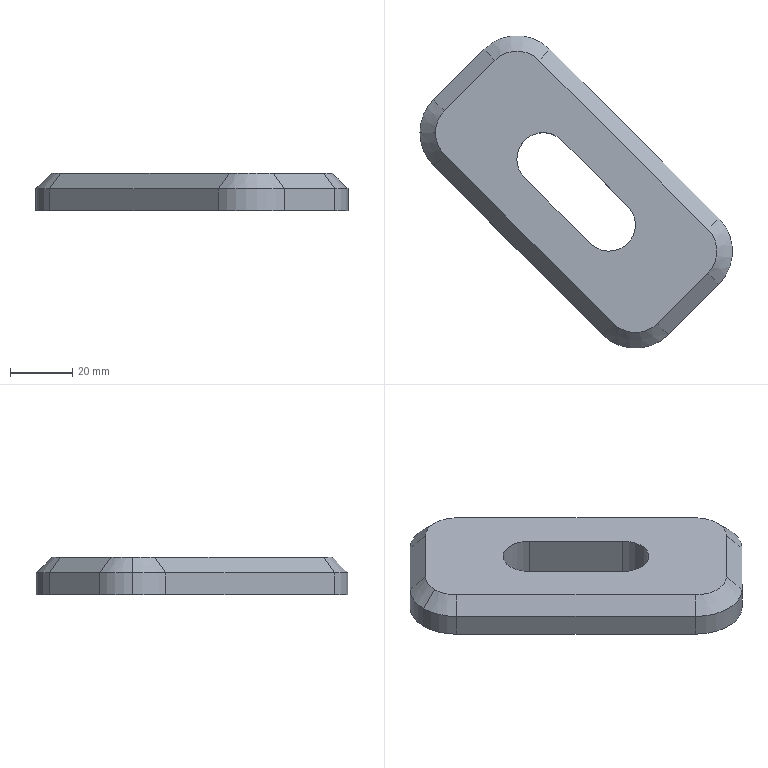Part | SolidWorks | features Chamfer 1, FlatPattern 1, SMBaseFlange 1, SheetMetal 1 | 1 solid | 25 faces | box 100.711 x 100.711 x 12 mm | volume 53343 mm3 | plane 12 | cylinder 8 | cone 5 | commonest cylinder face diameters 30 x5 17 x3
STEP:
#1=CARTESIAN_POINT('',(-96.355,309.376,12.));
#2=VERTEX_POINT('',#1);
#3=CARTESIAN_POINT('',(-93.426,302.305,12.));
#4=VERTEX_POINT('',#3);
#5=CARTESIAN_POINT('',(-86.355,309.376,12.));
#6=DIRECTION('',(0.,0.,1.));
#7=DIRECTION('',(-1.,0.,0.));
#8=AXIS2_PLACEMENT_3D('',#5,#6,#7);
#9=CIRCLE('',#8,10.);
#10=EDGE_CURVE('',#2,#4,#9,.T.);
#11=ORIENTED_EDGE('',*,*,#10,.F.);
#12=CARTESIAN_POINT('',(-101.355,309.376,7.));
#13=VERTEX_POINT('',#12);
#14=CARTESIAN_POINT('',(-96.355,309.376,12.));
#15=DIRECTION('',(-0.7071,0.,-0.7071));
#16=VECTOR('',#15,1000.);
#17=LINE('',#14,#16);
#18=EDGE_CURVE('',#2,#13,#17,.T.);
#19=ORIENTED_EDGE('',*,*,#18,.T.);
#20=CARTESIAN_POINT('',(-96.962,298.77,7.));
#21=VERTEX_POINT('',#20);
#22=CARTESIAN_POINT('',(-86.355,309.376,7.));
#23=DIRECTION('',(0.,0.,-1.));
#24=DIRECTION('',(-1.,0.,0.));
#25=AXIS2_PLACEMENT_3D('',#22,#23,#24);
#26=CIRCLE('',#25,15.);
#27=EDGE_CURVE('',#21,#13,#26,.T.);
#28=ORIENTED_EDGE('',*,*,#27,.F.);
#29=CARTESIAN_POINT('',(-96.962,298.77,7.));
#30=DIRECTION('',(0.5,0.5,0.7071));
#31=VECTOR('',#30,1000.);
#32=LINE('',#29,#31);
#33=EDGE_CURVE('',#21,#4,#32,.T.);
#34=ORIENTED_EDGE('',*,*,#33,.T.);
#35=EDGE_LOOP('',(#11,#19,#28,#34));
#36=FACE_OUTER_BOUND('',#35,.T.);
#37=CARTESIAN_POINT('',(-86.355,309.376,12.));
#38=DIRECTION('',(0.,0.,-1.));
#39=DIRECTION('',(-1.,0.,0.));
#40=AXIS2_PLACEMENT_3D('',#37,#38,#39);
#41=CONICAL_SURFACE('',#40,10.,0.7854);
#42=ADVANCED_FACE('',(#36),#41,.T.);
#43=CARTESIAN_POINT('',(-55.596,306.901,12.));
#44=VERTEX_POINT('',#43);
#45=CARTESIAN_POINT('',(-70.107,300.891,12.));
#46=VERTEX_POINT('',#45);
#47=CARTESIAN_POINT('',(-61.607,300.891,12.));
#48=DIRECTION('',(0.,0.,1.));
#49=DIRECTION('',(1.,0.,0.));
#50=AXIS2_PLACEMENT_3D('',#47,#48,#49);
#51=CIRCLE('',#50,8.5);
#52=EDGE_CURVE('',#44,#46,#51,.T.);
#53=ORIENTED_EDGE('',*,*,#52,.T.);
#54=CARTESIAN_POINT('',(-70.107,300.891,0.));
#55=VERTEX_POINT('',#54);
#56=CARTESIAN_POINT('',(-70.107,300.891,12.));
#57=DIRECTION('',(0.,0.,-1.));
#58=VECTOR('',#57,1000.);
#59=LINE('',#56,#58);
#60=EDGE_CURVE('',#46,#55,#59,.T.);
#61=ORIENTED_EDGE('',*,*,#60,.T.);
#62=CARTESIAN_POINT('',(-55.596,306.901,0.));
#63=VERTEX_POINT('',#62);
#64=CARTESIAN_POINT('',(-61.607,300.891,0.));
#65=DIRECTION('',(0.,0.,1.));
#66=DIRECTION('',(1.,0.,0.));
#67=AXIS2_PLACEMENT_3D('',#64,#65,#66);
#68=CIRCLE('',#67,8.5);
#69=EDGE_CURVE('',#63,#55,#68,.T.);
#70=ORIENTED_EDGE('',*,*,#69,.F.);
#71=CARTESIAN_POINT('',(-55.596,306.901,12.));
#72=DIRECTION('',(0.,0.,-1.));
#73=VECTOR('',#72,1000.);
#74=LINE('',#71,#73);
#75=EDGE_CURVE('',#44,#63,#74,.T.);
#76=ORIENTED_EDGE('',*,*,#75,.F.);
#77=EDGE_LOOP('',(#53,#61,#70,#76));
#78=FACE_OUTER_BOUND('',#77,.T.);
#79=CARTESIAN_POINT('',(-61.607,300.891,12.));
#80=DIRECTION('',(0.,0.,-1.));
#81=DIRECTION('',(-1.,0.,0.));
#82=AXIS2_PLACEMENT_3D('',#79,#80,#81);
#83=CYLINDRICAL_SURFACE('',#82,8.5);
#84=ADVANCED_FACE('',(#78),#83,.F.);
#85=ORIENTED_EDGE('',*,*,#27,.T.);
#86=CARTESIAN_POINT('',(-101.355,309.376,0.));
#87=VERTEX_POINT('',#86);
#88=CARTESIAN_POINT('',(-101.355,309.376,12.));
#89=DIRECTION('',(0.,0.,-1.));
#90=VECTOR('',#89,1000.);
#91=LINE('',#88,#90);
#92=EDGE_CURVE('',#13,#87,#91,.T.);
#93=ORIENTED_EDGE('',*,*,#92,.T.);
#94=CARTESIAN_POINT('',(-96.962,298.77,0.));
#95=VERTEX_POINT('',#94);
#96=CARTESIAN_POINT('',(-86.355,309.376,0.));
#97=DIRECTION('',(0.,0.,1.));
#98=DIRECTION('',(-1.,0.,0.));
#99=AXIS2_PLACEMENT_3D('',#96,#97,#98);
#100=CIRCLE('',#99,15.);
#101=EDGE_CURVE('',#87,#95,#100,.T.);
#102=ORIENTED_EDGE('',*,*,#101,.T.);
#103=CARTESIAN_POINT('',(-96.962,298.77,12.));
#104=DIRECTION('',(0.,0.,-1.));
#105=VECTOR('',#104,1000.);
#106=LINE('',#103,#105);
#107=EDGE_CURVE('',#21,#95,#106,.T.);
#108=ORIENTED_EDGE('',*,*,#107,.F.);
#109=EDGE_LOOP('',(#85,#93,#102,#108));
#110=FACE_OUTER_BOUND('',#109,.T.);
#111=CARTESIAN_POINT('',(-86.355,309.376,12.));
#112=DIRECTION('',(0.,0.,-1.));
#113=DIRECTION('',(-1.,0.,0.));
#114=AXIS2_PLACEMENT_3D('',#111,#112,#113);
#115=CYLINDRICAL_SURFACE('',#114,15.);
#116=ADVANCED_FACE('',(#110),#115,.T.);
#117=CARTESIAN_POINT('',(-8.574,264.121,12.));
#118=VERTEX_POINT('',#117);
#119=CARTESIAN_POINT('',(-8.574,278.263,12.));
#120=VERTEX_POINT('',#119);
#121=CARTESIAN_POINT('',(-15.645,271.192,12.));
#122=DIRECTION('',(0.,0.,1.));
#123=DIRECTION('',(-1.,0.,0.));
#124=AXIS2_PLACEMENT_3D('',#121,#122,#123);
#125=CIRCLE('',#124,10.);
#126=EDGE_CURVE('',#118,#120,#125,.T.);
#127=ORIENTED_EDGE('',*,*,#126,.T.);
#128=CARTESIAN_POINT('',(-63.021,332.711,12.));
#129=VERTEX_POINT('',#128);
#130=CARTESIAN_POINT('',(-8.574,278.263,12.));
#131=DIRECTION('',(-0.7071,0.7071,0.));
#132=VECTOR('',#131,1000.);
#133=LINE('',#130,#132);
#134=EDGE_CURVE('',#120,#129,#133,.T.);
#135=ORIENTED_EDGE('',*,*,#134,.T.);
#136=CARTESIAN_POINT('',(-77.163,332.711,12.));
#137=VERTEX_POINT('',#136);
#138=CARTESIAN_POINT('',(-70.092,325.64,12.));
#139=DIRECTION('',(0.,0.,1.));
#140=DIRECTION('',(-1.,0.,0.));
#141=AXIS2_PLACEMENT_3D('',#138,#139,#140);
#142=CIRCLE('',#141,10.);
#143=EDGE_CURVE('',#129,#137,#142,.T.);
#144=ORIENTED_EDGE('',*,*,#143,.T.);
#145=CARTESIAN_POINT('',(-93.426,316.447,12.));
#146=VERTEX_POINT('',#145);
#147=CARTESIAN_POINT('',(-77.163,332.711,12.));
#148=DIRECTION('',(-0.7071,-0.7071,0.));
#149=VECTOR('',#148,1000.);
#150=LINE('',#147,#149);
#151=EDGE_CURVE('',#137,#146,#150,.T.);
#152=ORIENTED_EDGE('',*,*,#151,.T.);
#153=CARTESIAN_POINT('',(-86.355,309.376,12.));
#154=DIRECTION('',(0.,0.,1.));
#155=DIRECTION('',(-1.,0.,0.));
#156=AXIS2_PLACEMENT_3D('',#153,#154,#155);
#157=CIRCLE('',#156,10.);
#158=EDGE_CURVE('',#146,#2,#157,.T.);
#159=ORIENTED_EDGE('',*,*,#158,.T.);
#160=ORIENTED_EDGE('',*,*,#10,.T.);
#161=CARTESIAN_POINT('',(-38.979,247.858,12.));
#162=VERTEX_POINT('',#161);
#163=CARTESIAN_POINT('',(-38.979,247.858,12.));
#164=DIRECTION('',(0.7071,-0.7071,0.));
#165=VECTOR('',#164,1000.);
#166=LINE('',#163,#165);
#167=EDGE_CURVE('',#4,#162,#166,.T.);
#168=ORIENTED_EDGE('',*,*,#167,.T.);
#169=CARTESIAN_POINT('',(-24.837,247.858,12.));
#170=VERTEX_POINT('',#169);
#171=CARTESIAN_POINT('',(-31.908,254.929,12.));
#172=DIRECTION('',(0.,0.,1.));
#173=DIRECTION('',(-1.,0.,0.));
#174=AXIS2_PLACEMENT_3D('',#171,#172,#173);
#175=CIRCLE('',#174,10.);
#176=EDGE_CURVE('',#162,#170,#175,.T.);
#177=ORIENTED_EDGE('',*,*,#176,.T.);
#178=CARTESIAN_POINT('',(-8.574,264.121,12.));
#179=DIRECTION('',(0.7071,0.7071,0.));
#180=VECTOR('',#179,1000.);
#181=LINE('',#178,#180);
#182=EDGE_CURVE('',#170,#118,#181,.T.);
#183=ORIENTED_EDGE('',*,*,#182,.T.);
#184=EDGE_LOOP('',(#127,#135,#144,#152,#159,#160,#168,#177,#183));
#185=FACE_OUTER_BOUND('',#184,.T.);
#186=CARTESIAN_POINT('',(-46.404,273.667,12.));
#187=VERTEX_POINT('',#186);
#188=CARTESIAN_POINT('',(-34.383,285.688,12.));
#189=VERTEX_POINT('',#188);
#190=CARTESIAN_POINT('',(-40.393,279.678,12.));
#191=DIRECTION('',(0.,0.,1.));
#192=DIRECTION('',(1.,0.,0.));
#193=AXIS2_PLACEMENT_3D('',#190,#191,#192);
#194=CIRCLE('',#193,8.5);
#195=EDGE_CURVE('',#187,#189,#194,.T.);
#196=ORIENTED_EDGE('',*,*,#195,.F.);
#197=CARTESIAN_POINT('',(-67.617,294.88,12.));
#198=VERTEX_POINT('',#197);
#199=CARTESIAN_POINT('',(-46.404,273.667,12.));
#200=DIRECTION('',(0.7071,-0.7071,0.));
#201=VECTOR('',#200,1000.);
#202=LINE('',#199,#201);
#203=EDGE_CURVE('',#198,#187,#202,.T.);
#204=ORIENTED_EDGE('',*,*,#203,.F.);
#205=CARTESIAN_POINT('',(-61.607,300.891,12.));
#206=DIRECTION('',(0.,0.,1.));
#207=DIRECTION('',(1.,0.,0.));
#208=AXIS2_PLACEMENT_3D('',#205,#206,#207);
#209=CIRCLE('',#208,8.5);
#210=EDGE_CURVE('',#46,#198,#209,.T.);
#211=ORIENTED_EDGE('',*,*,#210,.F.);
#212=ORIENTED_EDGE('',*,*,#52,.F.);
#213=CARTESIAN_POINT('',(-34.383,285.688,12.));
#214=DIRECTION('',(-0.7071,0.7071,0.));
#215=VECTOR('',#214,1000.);
#216=LINE('',#213,#215);
#217=EDGE_CURVE('',#189,#44,#216,.T.);
#218=ORIENTED_EDGE('',*,*,#217,.F.);
#219=EDGE_LOOP('',(#196,#204,#211,#212,#218));
#220=FACE_BOUND('',#219,.T.);
#221=CARTESIAN_POINT('',(-15.645,271.192,12.));
#222=DIRECTION('',(0.,0.,-1.));
#223=DIRECTION('',(-1.,0.,0.));
#224=AXIS2_PLACEMENT_3D('',#221,#222,#223);
#225=PLANE('',#224);
#226=ADVANCED_FACE('',(#185,#220),#225,.F.);
#227=CARTESIAN_POINT('',(-5.038,260.586,0.));
#228=VERTEX_POINT('',#227);
#229=CARTESIAN_POINT('',(-5.038,281.799,0.));
#230=VERTEX_POINT('',#229);
#231=CARTESIAN_POINT('',(-15.645,271.192,0.));
#232=DIRECTION('',(0.,0.,1.));
#233=DIRECTION('',(-1.,0.,0.));
#234=AXIS2_PLACEMENT_3D('',#231,#232,#233);
#235=CIRCLE('',#234,15.);
#236=EDGE_CURVE('',#228,#230,#235,.T.);
#237=ORIENTED_EDGE('',*,*,#236,.F.);
#238=CARTESIAN_POINT('',(-21.302,244.322,0.));
#239=VERTEX_POINT('',#238);
#240=CARTESIAN_POINT('',(-5.038,260.586,0.));
#241=DIRECTION('',(0.7071,0.7071,0.));
#242=VECTOR('',#241,1000.);
#243=LINE('',#240,#242);
#244=EDGE_CURVE('',#239,#228,#243,.T.);
#245=ORIENTED_EDGE('',*,*,#244,.F.);
#246=CARTESIAN_POINT('',(-42.515,244.322,0.));
#247=VERTEX_POINT('',#246);
#248=CARTESIAN_POINT('',(-31.908,254.929,0.));
#249=DIRECTION('',(0.,0.,1.));
#250=DIRECTION('',(-1.,0.,0.));
#251=AXIS2_PLACEMENT_3D('',#248,#249,#250);
#252=CIRCLE('',#251,15.);
#253=EDGE_CURVE('',#247,#239,#252,.T.);
#254=ORIENTED_EDGE('',*,*,#253,.F.);
#255=CARTESIAN_POINT('',(-42.515,244.322,0.));
#256=DIRECTION('',(0.7071,-0.7071,0.));
#257=VECTOR('',#256,1000.);
#258=LINE('',#255,#257);
#259=EDGE_CURVE('',#95,#247,#258,.T.);
#260=ORIENTED_EDGE('',*,*,#259,.F.);
#261=ORIENTED_EDGE('',*,*,#101,.F.);
#262=CARTESIAN_POINT('',(-96.962,319.983,0.));
#263=VERTEX_POINT('',#262);
#264=CARTESIAN_POINT('',(-86.355,309.376,0.));
#265=DIRECTION('',(0.,0.,1.));
#266=DIRECTION('',(-1.,0.,0.));
#267=AXIS2_PLACEMENT_3D('',#264,#265,#266);
#268=CIRCLE('',#267,15.);
#269=EDGE_CURVE('',#263,#87,#268,.T.);
#270=ORIENTED_EDGE('',*,*,#269,.F.);
#271=CARTESIAN_POINT('',(-80.698,336.246,0.));
#272=VERTEX_POINT('',#271);
#273=CARTESIAN_POINT('',(-96.962,319.983,0.));
#274=DIRECTION('',(-0.7071,-0.7071,0.));
#275=VECTOR('',#274,1000.);
#276=LINE('',#273,#275);
#277=EDGE_CURVE('',#272,#263,#276,.T.);
#278=ORIENTED_EDGE('',*,*,#277,.F.);
#279=CARTESIAN_POINT('',(-59.485,336.246,0.));
#280=VERTEX_POINT('',#279);
#281=CARTESIAN_POINT('',(-70.092,325.64,0.));
#282=DIRECTION('',(0.,0.,1.));
#283=DIRECTION('',(1.,0.,0.));
#284=AXIS2_PLACEMENT_3D('',#281,#282,#283);
#285=CIRCLE('',#284,15.);
#286=EDGE_CURVE('',#280,#272,#285,.T.);
#287=ORIENTED_EDGE('',*,*,#286,.F.);
#288=CARTESIAN_POINT('',(-59.485,336.246,0.));
#289=DIRECTION('',(-0.7071,0.7071,0.));
#290=VECTOR('',#289,1000.);
#291=LINE('',#288,#290);
#292=EDGE_CURVE('',#230,#280,#291,.T.);
#293=ORIENTED_EDGE('',*,*,#292,.F.);
#294=EDGE_LOOP('',(#237,#245,#254,#260,#261,#270,#278,#287,#293));
#295=FACE_OUTER_BOUND('',#294,.T.);
#296=CARTESIAN_POINT('',(-67.617,294.88,0.));
#297=VERTEX_POINT('',#296);
#298=CARTESIAN_POINT('',(-46.404,273.667,0.));
#299=VERTEX_POINT('',#298);
#300=CARTESIAN_POINT('',(-46.404,273.667,0.));
#301=DIRECTION('',(0.7071,-0.7071,0.));
#302=VECTOR('',#301,1000.);
#303=LINE('',#300,#302);
#304=EDGE_CURVE('',#297,#299,#303,.T.);
#305=ORIENTED_EDGE('',*,*,#304,.T.);
#306=CARTESIAN_POINT('',(-34.383,285.688,0.));
#307=VERTEX_POINT('',#306);
#308=CARTESIAN_POINT('',(-40.393,279.678,0.));
#309=DIRECTION('',(0.,0.,1.));
#310=DIRECTION('',(1.,0.,0.));
#311=AXIS2_PLACEMENT_3D('',#308,#309,#310);
#312=CIRCLE('',#311,8.5);
#313=EDGE_CURVE('',#299,#307,#312,.T.);
#314=ORIENTED_EDGE('',*,*,#313,.T.);
#315=CARTESIAN_POINT('',(-34.383,285.688,0.));
#316=DIRECTION('',(-0.7071,0.7071,0.));
#317=VECTOR('',#316,1000.);
#318=LINE('',#315,#317);
#319=EDGE_CURVE('',#307,#63,#318,.T.);
#320=ORIENTED_EDGE('',*,*,#319,.T.);
#321=ORIENTED_EDGE('',*,*,#69,.T.);
#322=CARTESIAN_POINT('',(-61.607,300.891,0.));
#323=DIRECTION('',(0.,0.,1.));
#324=DIRECTION('',(1.,0.,0.));
#325=AXIS2_PLACEMENT_3D('',#322,#323,#324);
#326=CIRCLE('',#325,8.5);
#327=EDGE_CURVE('',#55,#297,#326,.T.);
#328=ORIENTED_EDGE('',*,*,#327,.T.);
#329=EDGE_LOOP('',(#305,#314,#320,#321,#328));
#330=FACE_BOUND('',#329,.T.);
#331=CARTESIAN_POINT('',(-15.645,271.192,0.));
#332=DIRECTION('',(0.,0.,-1.));
#333=DIRECTION('',(-1.,0.,0.));
#334=AXIS2_PLACEMENT_3D('',#331,#332,#333);
#335=PLANE('',#334);
#336=ADVANCED_FACE('',(#295,#330),#335,.T.);
#337=CARTESIAN_POINT('',(-5.038,281.799,7.));
#338=VERTEX_POINT('',#337);
#339=CARTESIAN_POINT('',(-5.038,281.799,12.));
#340=DIRECTION('',(0.,0.,-1.));
#341=VECTOR('',#340,1000.);
#342=LINE('',#339,#341);
#343=EDGE_CURVE('',#338,#230,#342,.T.);
#344=ORIENTED_EDGE('',*,*,#343,.F.);
#345=CARTESIAN_POINT('',(-5.038,260.586,7.));
#346=VERTEX_POINT('',#345);
#347=CARTESIAN_POINT('',(-15.645,271.192,7.));
#348=DIRECTION('',(0.,0.,-1.));
#349=DIRECTION('',(-1.,0.,0.));
#350=AXIS2_PLACEMENT_3D('',#347,#348,#349);
#351=CIRCLE('',#350,15.);
#352=EDGE_CURVE('',#338,#346,#351,.T.);
#353=ORIENTED_EDGE('',*,*,#352,.T.);
#354=CARTESIAN_POINT('',(-5.038,260.586,12.));
#355=DIRECTION('',(0.,0.,-1.));
#356=VECTOR('',#355,1000.);
#357=LINE('',#354,#356);
#358=EDGE_CURVE('',#346,#228,#357,.T.);
#359=ORIENTED_EDGE('',*,*,#358,.T.);
#360=ORIENTED_EDGE('',*,*,#236,.T.);
#361=EDGE_LOOP('',(#344,#353,#359,#360));
#362=FACE_OUTER_BOUND('',#361,.T.);
#363=CARTESIAN_POINT('',(-15.645,271.192,12.));
#364=DIRECTION('',(0.,0.,-1.));
#365=DIRECTION('',(-1.,0.,0.));
#366=AXIS2_PLACEMENT_3D('',#363,#364,#365);
#367=CYLINDRICAL_SURFACE('',#366,15.);
#368=ADVANCED_FACE('',(#362),#367,.T.);
#369=CARTESIAN_POINT('',(-59.485,336.246,7.));
#370=VERTEX_POINT('',#369);
#371=CARTESIAN_POINT('',(-59.485,336.246,12.));
#372=DIRECTION('',(0.,0.,-1.));
#373=VECTOR('',#372,1000.);
#374=LINE('',#371,#373);
#375=EDGE_CURVE('',#370,#280,#374,.T.);
#376=ORIENTED_EDGE('',*,*,#375,.F.);
#377=CARTESIAN_POINT('',(-59.485,336.246,7.));
#378=DIRECTION('',(0.7071,-0.7071,0.));
#379=VECTOR('',#378,1000.);
#380=LINE('',#377,#379);
#381=EDGE_CURVE('',#370,#338,#380,.T.);
#382=ORIENTED_EDGE('',*,*,#381,.T.);
#383=ORIENTED_EDGE('',*,*,#343,.T.);
#384=ORIENTED_EDGE('',*,*,#292,.T.);
#385=EDGE_LOOP('',(#376,#382,#383,#384));
#386=FACE_OUTER_BOUND('',#385,.T.);
#387=CARTESIAN_POINT('',(-59.485,336.246,12.));
#388=DIRECTION('',(-0.7071,-0.7071,0.));
#389=DIRECTION('',(0.7071,-0.7071,0.));
#390=AXIS2_PLACEMENT_3D('',#387,#388,#389);
#391=PLANE('',#390);
#392=ADVANCED_FACE('',(#386),#391,.F.);
#393=CARTESIAN_POINT('',(-80.698,336.246,7.));
#394=VERTEX_POINT('',#393);
#395=CARTESIAN_POINT('',(-80.698,336.246,12.));
#396=DIRECTION('',(0.,0.,-1.));
#397=VECTOR('',#396,1000.);
#398=LINE('',#395,#397);
#399=EDGE_CURVE('',#394,#272,#398,.T.);
#400=ORIENTED_EDGE('',*,*,#399,.F.);
#401=CARTESIAN_POINT('',(-70.092,325.64,7.));
#402=DIRECTION('',(0.,0.,-1.));
#403=DIRECTION('',(-1.,0.,0.));
#404=AXIS2_PLACEMENT_3D('',#401,#402,#403);
#405=CIRCLE('',#404,15.);
#406=EDGE_CURVE('',#394,#370,#405,.T.);
#407=ORIENTED_EDGE('',*,*,#406,.T.);
#408=ORIENTED_EDGE('',*,*,#375,.T.);
#409=ORIENTED_EDGE('',*,*,#286,.T.);
#410=EDGE_LOOP('',(#400,#407,#408,#409));
#411=FACE_OUTER_BOUND('',#410,.T.);
#412=CARTESIAN_POINT('',(-70.092,325.64,12.));
#413=DIRECTION('',(0.,0.,-1.));
#414=DIRECTION('',(-1.,0.,0.));
#415=AXIS2_PLACEMENT_3D('',#412,#413,#414);
#416=CYLINDRICAL_SURFACE('',#415,15.);
#417=ADVANCED_FACE('',(#411),#416,.T.);
#418=CARTESIAN_POINT('',(-96.962,319.983,7.));
#419=VERTEX_POINT('',#418);
#420=CARTESIAN_POINT('',(-96.962,319.983,12.));
#421=DIRECTION('',(0.,0.,-1.));
#422=VECTOR('',#421,1000.);
#423=LINE('',#420,#422);
#424=EDGE_CURVE('',#419,#263,#423,.T.);
#425=ORIENTED_EDGE('',*,*,#424,.F.);
#426=CARTESIAN_POINT('',(-96.962,319.983,7.));
#427=DIRECTION('',(0.7071,0.7071,0.));
#428=VECTOR('',#427,1000.);
#429=LINE('',#426,#428);
#430=EDGE_CURVE('',#419,#394,#429,.T.);
#431=ORIENTED_EDGE('',*,*,#430,.T.);
#432=ORIENTED_EDGE('',*,*,#399,.T.);
#433=ORIENTED_EDGE('',*,*,#277,.T.);
#434=EDGE_LOOP('',(#425,#431,#432,#433));
#435=FACE_OUTER_BOUND('',#434,.T.);
#436=CARTESIAN_POINT('',(-96.962,319.983,12.));
#437=DIRECTION('',(0.7071,-0.7071,0.));
#438=DIRECTION('',(0.7071,0.7071,0.));
#439=AXIS2_PLACEMENT_3D('',#436,#437,#438);
#440=PLANE('',#439);
#441=ADVANCED_FACE('',(#435),#440,.F.);
#442=ORIENTED_EDGE('',*,*,#92,.F.);
#443=CARTESIAN_POINT('',(-86.355,309.376,7.));
#444=DIRECTION('',(0.,0.,-1.));
#445=DIRECTION('',(-1.,0.,0.));
#446=AXIS2_PLACEMENT_3D('',#443,#444,#445);
#447=CIRCLE('',#446,15.);
#448=EDGE_CURVE('',#13,#419,#447,.T.);
#449=ORIENTED_EDGE('',*,*,#448,.T.);
#450=ORIENTED_EDGE('',*,*,#424,.T.);
#451=ORIENTED_EDGE('',*,*,#269,.T.);
#452=EDGE_LOOP('',(#442,#449,#450,#451));
#453=FACE_OUTER_BOUND('',#452,.T.);
#454=CARTESIAN_POINT('',(-86.355,309.376,12.));
#455=DIRECTION('',(0.,0.,-1.));
#456=DIRECTION('',(-1.,0.,0.));
#457=AXIS2_PLACEMENT_3D('',#454,#455,#456);
#458=CYLINDRICAL_SURFACE('',#457,15.);
#459=ADVANCED_FACE('',(#453),#458,.T.);
#460=CARTESIAN_POINT('',(-42.515,244.322,7.));
#461=VERTEX_POINT('',#460);
#462=CARTESIAN_POINT('',(-42.515,244.322,12.));
#463=DIRECTION('',(0.,0.,-1.));
#464=VECTOR('',#463,1000.);
#465=LINE('',#462,#464);
#466=EDGE_CURVE('',#461,#247,#465,.T.);
#467=ORIENTED_EDGE('',*,*,#466,.F.);
#468=CARTESIAN_POINT('',(-42.515,244.322,7.));
#469=DIRECTION('',(-0.7071,0.7071,0.));
#470=VECTOR('',#469,1000.);
#471=LINE('',#468,#470);
#472=EDGE_CURVE('',#461,#21,#471,.T.);
#473=ORIENTED_EDGE('',*,*,#472,.T.);
#474=ORIENTED_EDGE('',*,*,#107,.T.);
#475=ORIENTED_EDGE('',*,*,#259,.T.);
#476=EDGE_LOOP('',(#467,#473,#474,#475));
#477=FACE_OUTER_BOUND('',#476,.T.);
#478=CARTESIAN_POINT('',(-42.515,244.322,12.));
#479=DIRECTION('',(0.7071,0.7071,0.));
#480=DIRECTION('',(-0.7071,0.7071,0.));
#481=AXIS2_PLACEMENT_3D('',#478,#479,#480);
#482=PLANE('',#481);
#483=ADVANCED_FACE('',(#477),#482,.F.);
#484=CARTESIAN_POINT('',(-21.302,244.322,7.));
#485=VERTEX_POINT('',#484);
#486=CARTESIAN_POINT('',(-21.302,244.322,12.));
#487=DIRECTION('',(0.,0.,-1.));
#488=VECTOR('',#487,1000.);
#489=LINE('',#486,#488);
#490=EDGE_CURVE('',#485,#239,#489,.T.);
#491=ORIENTED_EDGE('',*,*,#490,.F.);
#492=CARTESIAN_POINT('',(-31.908,254.929,7.));
#493=DIRECTION('',(0.,0.,-1.));
#494=DIRECTION('',(-1.,0.,0.));
#495=AXIS2_PLACEMENT_3D('',#492,#493,#494);
#496=CIRCLE('',#495,15.);
#497=EDGE_CURVE('',#485,#461,#496,.T.);
#498=ORIENTED_EDGE('',*,*,#497,.T.);
#499=ORIENTED_EDGE('',*,*,#466,.T.);
#500=ORIENTED_EDGE('',*,*,#253,.T.);
#501=EDGE_LOOP('',(#491,#498,#499,#500));
#502=FACE_OUTER_BOUND('',#501,.T.);
#503=CARTESIAN_POINT('',(-31.908,254.929,12.));
#504=DIRECTION('',(0.,0.,-1.));
#505=DIRECTION('',(-1.,0.,0.));
#506=AXIS2_PLACEMENT_3D('',#503,#504,#505);
#507=CYLINDRICAL_SURFACE('',#506,15.);
#508=ADVANCED_FACE('',(#502),#507,.T.);
#509=ORIENTED_EDGE('',*,*,#358,.F.);
#510=CARTESIAN_POINT('',(-5.038,260.586,7.));
#511=DIRECTION('',(-0.7071,-0.7071,0.));
#512=VECTOR('',#511,1000.);
#513=LINE('',#510,#512);
#514=EDGE_CURVE('',#346,#485,#513,.T.);
#515=ORIENTED_EDGE('',*,*,#514,.T.);
#516=ORIENTED_EDGE('',*,*,#490,.T.);
#517=ORIENTED_EDGE('',*,*,#244,.T.);
#518=EDGE_LOOP('',(#509,#515,#516,#517));
#519=FACE_OUTER_BOUND('',#518,.T.);
#520=CARTESIAN_POINT('',(-5.038,260.586,12.));
#521=DIRECTION('',(-0.7071,0.7071,0.));
#522=DIRECTION('',(-0.7071,-0.7071,0.));
#523=AXIS2_PLACEMENT_3D('',#520,#521,#522);
#524=PLANE('',#523);
#525=ADVANCED_FACE('',(#519),#524,.F.);
#526=ORIENTED_EDGE('',*,*,#313,.F.);
#527=CARTESIAN_POINT('',(-46.404,273.667,12.));
#528=DIRECTION('',(0.,0.,-1.));
#529=VECTOR('',#528,1000.);
#530=LINE('',#527,#529);
#531=EDGE_CURVE('',#187,#299,#530,.T.);
#532=ORIENTED_EDGE('',*,*,#531,.F.);
#533=ORIENTED_EDGE('',*,*,#195,.T.);
#534=CARTESIAN_POINT('',(-34.383,285.688,12.));
#535=DIRECTION('',(0.,0.,-1.));
#536=VECTOR('',#535,1000.);
#537=LINE('',#534,#536);
#538=EDGE_CURVE('',#189,#307,#537,.T.);
#539=ORIENTED_EDGE('',*,*,#538,.T.);
#540=EDGE_LOOP('',(#526,#532,#533,#539));
#541=FACE_OUTER_BOUND('',#540,.T.);
#542=CARTESIAN_POINT('',(-40.393,279.678,12.));
#543=DIRECTION('',(0.,0.,-1.));
#544=DIRECTION('',(-1.,0.,0.));
#545=AXIS2_PLACEMENT_3D('',#542,#543,#544);
#546=CYLINDRICAL_SURFACE('',#545,8.5);
#547=ADVANCED_FACE('',(#541),#546,.F.);
#548=ORIENTED_EDGE('',*,*,#319,.F.);
#549=ORIENTED_EDGE('',*,*,#538,.F.);
#550=ORIENTED_EDGE('',*,*,#217,.T.);
#551=ORIENTED_EDGE('',*,*,#75,.T.);
#552=EDGE_LOOP('',(#548,#549,#550,#551));
#553=FACE_OUTER_BOUND('',#552,.T.);
#554=CARTESIAN_POINT('',(-34.383,285.688,12.));
#555=DIRECTION('',(-0.7071,-0.7071,0.));
#556=DIRECTION('',(0.7071,-0.7071,0.));
#557=AXIS2_PLACEMENT_3D('',#554,#555,#556);
#558=PLANE('',#557);
#559=ADVANCED_FACE('',(#553),#558,.T.);
#560=ORIENTED_EDGE('',*,*,#60,.F.);
#561=ORIENTED_EDGE('',*,*,#210,.T.);
#562=CARTESIAN_POINT('',(-67.617,294.88,12.));
#563=DIRECTION('',(0.,0.,-1.));
#564=VECTOR('',#563,1000.);
#565=LINE('',#562,#564);
#566=EDGE_CURVE('',#198,#297,#565,.T.);
#567=ORIENTED_EDGE('',*,*,#566,.T.);
#568=ORIENTED_EDGE('',*,*,#327,.F.);
#569=EDGE_LOOP('',(#560,#561,#567,#568));
#570=FACE_OUTER_BOUND('',#569,.T.);
#571=CARTESIAN_POINT('',(-61.607,300.891,12.));
#572=DIRECTION('',(0.,0.,-1.));
#573=DIRECTION('',(-1.,0.,0.));
#574=AXIS2_PLACEMENT_3D('',#571,#572,#573);
#575=CYLINDRICAL_SURFACE('',#574,8.5);
#576=ADVANCED_FACE('',(#570),#575,.F.);
#577=ORIENTED_EDGE('',*,*,#304,.F.);
#578=ORIENTED_EDGE('',*,*,#566,.F.);
#579=ORIENTED_EDGE('',*,*,#203,.T.);
#580=ORIENTED_EDGE('',*,*,#531,.T.);
#581=EDGE_LOOP('',(#577,#578,#579,#580));
#582=FACE_OUTER_BOUND('',#581,.T.);
#583=CARTESIAN_POINT('',(-46.404,273.667,12.));
#584=DIRECTION('',(0.7071,0.7071,0.));
#585=DIRECTION('',(-0.7071,0.7071,0.));
#586=AXIS2_PLACEMENT_3D('',#583,#584,#585);
#587=PLANE('',#586);
#588=ADVANCED_FACE('',(#582),#587,.T.);
#589=ORIENTED_EDGE('',*,*,#33,.F.);
#590=ORIENTED_EDGE('',*,*,#472,.F.);
#591=CARTESIAN_POINT('',(-38.979,247.858,12.));
#592=DIRECTION('',(-0.5,-0.5,-0.7071));
#593=VECTOR('',#592,1000.);
#594=LINE('',#591,#593);
#595=EDGE_CURVE('',#162,#461,#594,.T.);
#596=ORIENTED_EDGE('',*,*,#595,.F.);
#597=ORIENTED_EDGE('',*,*,#167,.F.);
#598=EDGE_LOOP('',(#589,#590,#596,#597));
#599=FACE_OUTER_BOUND('',#598,.T.);
#600=CARTESIAN_POINT('',(-38.979,247.858,12.));
#601=DIRECTION('',(0.5,0.5,-0.7071));
#602=DIRECTION('',(0.7071,-0.7071,0.));
#603=AXIS2_PLACEMENT_3D('',#600,#601,#602);
#604=PLANE('',#603);
#605=ADVANCED_FACE('',(#599),#604,.F.);
#606=ORIENTED_EDGE('',*,*,#595,.T.);
#607=ORIENTED_EDGE('',*,*,#497,.F.);
#608=CARTESIAN_POINT('',(-24.837,247.858,12.));
#609=DIRECTION('',(0.5,-0.5,-0.7071));
#610=VECTOR('',#609,1000.);
#611=LINE('',#608,#610);
#612=EDGE_CURVE('',#170,#485,#611,.T.);
#613=ORIENTED_EDGE('',*,*,#612,.F.);
#614=ORIENTED_EDGE('',*,*,#176,.F.);
#615=EDGE_LOOP('',(#606,#607,#613,#614));
#616=FACE_OUTER_BOUND('',#615,.T.);
#617=CARTESIAN_POINT('',(-31.908,254.929,12.));
#618=DIRECTION('',(0.,0.,-1.));
#619=DIRECTION('',(-1.,0.,0.));
#620=AXIS2_PLACEMENT_3D('',#617,#618,#619);
#621=CONICAL_SURFACE('',#620,10.,0.7854);
#622=ADVANCED_FACE('',(#616),#621,.T.);
#623=ORIENTED_EDGE('',*,*,#18,.F.);
#624=ORIENTED_EDGE('',*,*,#158,.F.);
#625=CARTESIAN_POINT('',(-96.962,319.983,7.));
#626=DIRECTION('',(0.5,-0.5,0.7071));
#627=VECTOR('',#626,1000.);
#628=LINE('',#625,#627);
#629=EDGE_CURVE('',#419,#146,#628,.T.);
#630=ORIENTED_EDGE('',*,*,#629,.F.);
#631=ORIENTED_EDGE('',*,*,#448,.F.);
#632=EDGE_LOOP('',(#623,#624,#630,#631));
#633=FACE_OUTER_BOUND('',#632,.T.);
#634=CARTESIAN_POINT('',(-86.355,309.376,12.));
#635=DIRECTION('',(0.,0.,-1.));
#636=DIRECTION('',(-1.,0.,0.));
#637=AXIS2_PLACEMENT_3D('',#634,#635,#636);
#638=CONICAL_SURFACE('',#637,10.,0.7854);
#639=ADVANCED_FACE('',(#633),#638,.T.);
#640=ORIENTED_EDGE('',*,*,#612,.T.);
#641=ORIENTED_EDGE('',*,*,#514,.F.);
#642=CARTESIAN_POINT('',(-8.574,264.121,12.));
#643=DIRECTION('',(0.5,-0.5,-0.7071));
#644=VECTOR('',#643,1000.);
#645=LINE('',#642,#644);
#646=EDGE_CURVE('',#118,#346,#645,.T.);
#647=ORIENTED_EDGE('',*,*,#646,.F.);
#648=ORIENTED_EDGE('',*,*,#182,.F.);
#649=EDGE_LOOP('',(#640,#641,#647,#648));
#650=FACE_OUTER_BOUND('',#649,.T.);
#651=CARTESIAN_POINT('',(-8.574,264.121,12.));
#652=DIRECTION('',(-0.5,0.5,-0.7071));
#653=DIRECTION('',(0.7071,0.7071,0.));
#654=AXIS2_PLACEMENT_3D('',#651,#652,#653);
#655=PLANE('',#654);
#656=ADVANCED_FACE('',(#650),#655,.F.);
#657=ORIENTED_EDGE('',*,*,#629,.T.);
#658=ORIENTED_EDGE('',*,*,#151,.F.);
#659=CARTESIAN_POINT('',(-80.698,336.246,7.));
#660=DIRECTION('',(0.5,-0.5,0.7071));
#661=VECTOR('',#660,1000.);
#662=LINE('',#659,#661);
#663=EDGE_CURVE('',#394,#137,#662,.T.);
#664=ORIENTED_EDGE('',*,*,#663,.F.);
#665=ORIENTED_EDGE('',*,*,#430,.F.);
#666=EDGE_LOOP('',(#657,#658,#664,#665));
#667=FACE_OUTER_BOUND('',#666,.T.);
#668=CARTESIAN_POINT('',(-77.163,332.711,12.));
#669=DIRECTION('',(0.5,-0.5,-0.7071));
#670=DIRECTION('',(-0.7071,-0.7071,0.));
#671=AXIS2_PLACEMENT_3D('',#668,#669,#670);
#672=PLANE('',#671);
#673=ADVANCED_FACE('',(#667),#672,.F.);
#674=ORIENTED_EDGE('',*,*,#646,.T.);
#675=ORIENTED_EDGE('',*,*,#352,.F.);
#676=CARTESIAN_POINT('',(-8.574,278.263,12.));
#677=DIRECTION('',(0.5,0.5,-0.7071));
#678=VECTOR('',#677,1000.);
#679=LINE('',#676,#678);
#680=EDGE_CURVE('',#120,#338,#679,.T.);
#681=ORIENTED_EDGE('',*,*,#680,.F.);
#682=ORIENTED_EDGE('',*,*,#126,.F.);
#683=EDGE_LOOP('',(#674,#675,#681,#682));
#684=FACE_OUTER_BOUND('',#683,.T.);
#685=CARTESIAN_POINT('',(-15.645,271.192,12.));
#686=DIRECTION('',(0.,0.,-1.));
#687=DIRECTION('',(-1.,0.,0.));
#688=AXIS2_PLACEMENT_3D('',#685,#686,#687);
#689=CONICAL_SURFACE('',#688,10.,0.7854);
#690=ADVANCED_FACE('',(#684),#689,.T.);
#691=ORIENTED_EDGE('',*,*,#663,.T.);
#692=ORIENTED_EDGE('',*,*,#143,.F.);
#693=CARTESIAN_POINT('',(-59.485,336.246,7.));
#694=DIRECTION('',(-0.5,-0.5,0.7071));
#695=VECTOR('',#694,1000.);
#696=LINE('',#693,#695);
#697=EDGE_CURVE('',#370,#129,#696,.T.);
#698=ORIENTED_EDGE('',*,*,#697,.F.);
#699=ORIENTED_EDGE('',*,*,#406,.F.);
#700=EDGE_LOOP('',(#691,#692,#698,#699));
#701=FACE_OUTER_BOUND('',#700,.T.);
#702=CARTESIAN_POINT('',(-70.092,325.64,12.));
#703=DIRECTION('',(0.,0.,-1.));
#704=DIRECTION('',(-1.,0.,0.));
#705=AXIS2_PLACEMENT_3D('',#702,#703,#704);
#706=CONICAL_SURFACE('',#705,10.,0.7854);
#707=ADVANCED_FACE('',(#701),#706,.T.);
#708=ORIENTED_EDGE('',*,*,#680,.T.);
#709=ORIENTED_EDGE('',*,*,#381,.F.);
#710=ORIENTED_EDGE('',*,*,#697,.T.);
#711=ORIENTED_EDGE('',*,*,#134,.F.);
#712=EDGE_LOOP('',(#708,#709,#710,#711));
#713=FACE_OUTER_BOUND('',#712,.T.);
#714=CARTESIAN_POINT('',(-8.574,278.263,12.));
#715=DIRECTION('',(-0.5,-0.5,-0.7071));
#716=DIRECTION('',(-0.7071,0.7071,0.));
#717=AXIS2_PLACEMENT_3D('',#714,#715,#716);
#718=PLANE('',#717);
#719=ADVANCED_FACE('',(#713),#718,.F.);
#720=CLOSED_SHELL('',(#42,#84,#116,#226,#336,#368,#392,#417,#441,#459,#483,#508,#525,#547,#559,#576,#588,#605,#622,#639,#656,#673,#690,#707,#719));
#721=MANIFOLD_SOLID_BREP('',#720);
#722=CARTESIAN_POINT('',(0.,0.,0.));
#723=DIRECTION('',(0.,0.,1.));
#724=DIRECTION('',(1.,0.,0.));
#725=AXIS2_PLACEMENT_3D('',#722,#723,#724);
#726=(LENGTH_UNIT()NAMED_UNIT(*)SI_UNIT(.MILLI.,.METRE.));
#727=UNCERTAINTY_MEASURE_WITH_UNIT(LENGTH_MEASURE(0.00001),#726,'','');
#728=(NAMED_UNIT(*)PLANE_ANGLE_UNIT()SI_UNIT($,.RADIAN.));
#729=(NAMED_UNIT(*)SI_UNIT($,.STERADIAN.)SOLID_ANGLE_UNIT());
#730=(GEOMETRIC_REPRESENTATION_CONTEXT(3)GLOBAL_UNCERTAINTY_ASSIGNED_CONTEXT((#727))GLOBAL_UNIT_ASSIGNED_CONTEXT((#726,#728,#729))REPRESENTATION_CONTEXT('',''));
#731=ADVANCED_BREP_SHAPE_REPRESENTATION('',(#721,#725),#730);